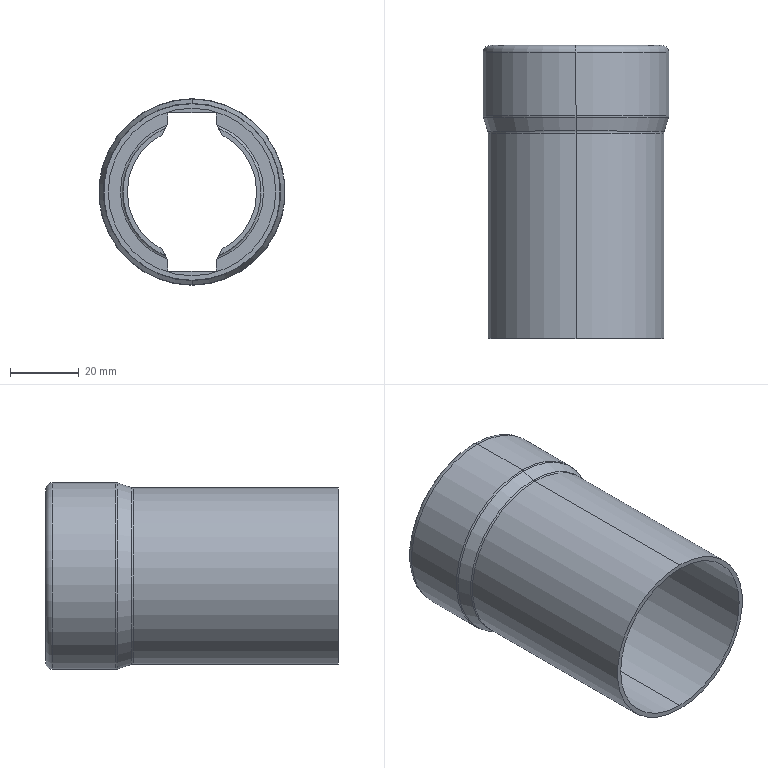Part | SolidWorks | features BaseBody 1 | 1 solid | 47 faces | box 54.2 x 85.2 x 54.2 mm | volume 19561 mm3 | torus 16 | plane 15 | cylinder 12 | cone 4 | commonest cylinder face diameters 37.6 x2 40.2 x2 48.7 x2 51.3 x2 51.6 x2 54.2 x2